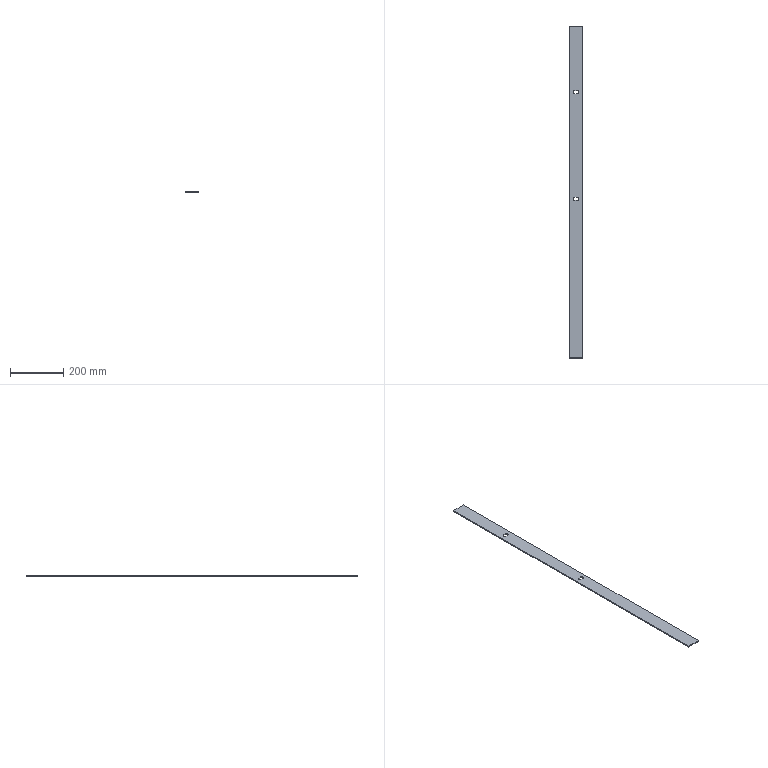Part | STEP file | E3-护栏加固Plate 1 | 1 solid | 16 faces | box 52 x 1250 x 4 mm | volume 258135 mm3 | plane 10 | cylinder 6 | commonest cylinder face diameters 12 x6
STEP:
#1=CARTESIAN_POINT('',(0.,0.,0.));
#2=DIRECTION('',(0.,0.,1.));
#3=DIRECTION('',(1.,0.,0.));
#4=AXIS2_PLACEMENT_3D('',#1,#2,#3);
#5=CARTESIAN_POINT('',(5.,369.,-4.));
#6=VERTEX_POINT('',#5);
#7=CARTESIAN_POINT('',(5.,369.,0.));
#8=VERTEX_POINT('',#7);
#9=CARTESIAN_POINT('',(5.,369.,-4.));
#10=DIRECTION('',(0.,0.,1.));
#11=VECTOR('',#10,1.);
#12=LINE('',#9,#11);
#13=CARTESIAN_POINT('',(5.,375.,-4.));
#14=DIRECTION('',(0.,0.,-1.));
#15=DIRECTION('',(1.,0.,0.));
#16=AXIS2_PLACEMENT_3D('',#13,#14,#15);
#17=CYLINDRICAL_SURFACE('',#16,6.);
#18=CARTESIAN_POINT('',(1.571,0.));
#19=DIRECTION('',(0.,-1.));
#20=VECTOR('',#19,1.);
#21=LINE('',#18,#20);
#22=(GEOMETRIC_REPRESENTATION_CONTEXT(2)PARAMETRIC_REPRESENTATION_CONTEXT()REPRESENTATION_CONTEXT('',''));
#23=DEFINITIONAL_REPRESENTATION('',(#21),#22);
#24=PCURVE('',#17,#23);
#25=CARTESIAN_POINT('',(-5.,369.,-4.));
#26=DIRECTION('',(0.,-1.,0.));
#27=DIRECTION('',(0.,0.,1.));
#28=AXIS2_PLACEMENT_3D('',#25,#26,#27);
#29=PLANE('',#28);
#30=CARTESIAN_POINT('',(0.,-10.));
#31=DIRECTION('',(1.,0.));
#32=VECTOR('',#31,1.);
#33=LINE('',#30,#32);
#34=(GEOMETRIC_REPRESENTATION_CONTEXT(2)PARAMETRIC_REPRESENTATION_CONTEXT()REPRESENTATION_CONTEXT('',''));
#35=DEFINITIONAL_REPRESENTATION('',(#33),#34);
#36=PCURVE('',#29,#35);
#37=SURFACE_CURVE('',#12,(#24,#36),.PCURVE_S1.);
#38=EDGE_CURVE('',#6,#8,#37,.T.);
#39=ORIENTED_EDGE('',*,*,#38,.F.);
#40=CARTESIAN_POINT('',(11.,375.,-4.));
#41=VERTEX_POINT('',#40);
#42=CARTESIAN_POINT('',(5.,375.,-4.));
#43=DIRECTION('',(0.,0.,1.));
#44=DIRECTION('',(1.,0.,0.));
#45=AXIS2_PLACEMENT_3D('',#42,#43,#44);
#46=CIRCLE('',#45,6.);
#47=CARTESIAN_POINT('',(6.283,0.));
#48=DIRECTION('',(-1.,0.));
#49=VECTOR('',#48,1.);
#50=LINE('',#47,#49);
#51=(GEOMETRIC_REPRESENTATION_CONTEXT(2)PARAMETRIC_REPRESENTATION_CONTEXT()REPRESENTATION_CONTEXT('',''));
#52=DEFINITIONAL_REPRESENTATION('',(#50),#51);
#53=PCURVE('',#17,#52);
#54=CARTESIAN_POINT('',(0.,0.,-4.));
#55=DIRECTION('',(0.,0.,-1.));
#56=DIRECTION('',(1.,0.,0.));
#57=AXIS2_PLACEMENT_3D('',#54,#55,#56);
#58=PLANE('',#57);
#59=CARTESIAN_POINT('',(11.,-375.));
#60=CARTESIAN_POINT('',(11.,-385.392));
#61=CARTESIAN_POINT('',(2.,-380.196));
#62=CARTESIAN_POINT('',(-7.,-375.));
#63=CARTESIAN_POINT('',(2.,-369.804));
#64=CARTESIAN_POINT('',(11.,-364.608));
#65=CARTESIAN_POINT('',(11.,-375.));
#66=(BOUNDED_CURVE()B_SPLINE_CURVE(2,(#59,#60,#61,#62,#63,#64,#65),.UNSPECIFIED.,.T.,.F.)B_SPLINE_CURVE_WITH_KNOTS((1,2,2,2,2,1),(-2.094,0.,2.094,4.189,6.283,8.378),.UNSPECIFIED.)CURVE()GEOMETRIC_REPRESENTATION_ITEM()RATIONAL_B_SPLINE_CURVE((1.,0.5,1.,0.5,1.,0.5,1.))REPRESENTATION_ITEM(''));
#67=(GEOMETRIC_REPRESENTATION_CONTEXT(2)PARAMETRIC_REPRESENTATION_CONTEXT()REPRESENTATION_CONTEXT('',''));
#68=DEFINITIONAL_REPRESENTATION('',(#66),#67);
#69=PCURVE('',#58,#68);
#70=SURFACE_CURVE('',#46,(#53,#69),.PCURVE_S1.);
#71=EDGE_CURVE('',#6,#41,#70,.T.);
#72=ORIENTED_EDGE('',*,*,#71,.T.);
#73=CARTESIAN_POINT('',(11.,375.,0.));
#74=VERTEX_POINT('',#73);
#75=CARTESIAN_POINT('',(11.,375.,-4.));
#76=DIRECTION('',(0.,0.,-1.));
#77=VECTOR('',#76,1.);
#78=LINE('',#75,#77);
#79=CARTESIAN_POINT('',(0.,0.));
#80=DIRECTION('',(0.,1.));
#81=VECTOR('',#80,1.);
#82=LINE('',#79,#81);
#83=(GEOMETRIC_REPRESENTATION_CONTEXT(2)PARAMETRIC_REPRESENTATION_CONTEXT()REPRESENTATION_CONTEXT('',''));
#84=DEFINITIONAL_REPRESENTATION('',(#82),#83);
#85=PCURVE('',#17,#84);
#86=CARTESIAN_POINT('',(5.,375.,-4.));
#87=DIRECTION('',(0.,0.,-1.));
#88=DIRECTION('',(1.,0.,0.));
#89=AXIS2_PLACEMENT_3D('',#86,#87,#88);
#90=CYLINDRICAL_SURFACE('',#89,6.);
#91=CARTESIAN_POINT('',(6.283,0.));
#92=DIRECTION('',(0.,1.));
#93=VECTOR('',#92,1.);
#94=LINE('',#91,#93);
#95=(GEOMETRIC_REPRESENTATION_CONTEXT(2)PARAMETRIC_REPRESENTATION_CONTEXT()REPRESENTATION_CONTEXT('',''));
#96=DEFINITIONAL_REPRESENTATION('',(#94),#95);
#97=PCURVE('',#90,#96);
#98=SURFACE_CURVE('',#78,(#85,#97),.PCURVE_S1.);
#99=EDGE_CURVE('',#74,#41,#98,.T.);
#100=ORIENTED_EDGE('',*,*,#99,.F.);
#101=CARTESIAN_POINT('',(5.,375.,0.));
#102=DIRECTION('',(0.,0.,1.));
#103=DIRECTION('',(1.,0.,0.));
#104=AXIS2_PLACEMENT_3D('',#101,#102,#103);
#105=CIRCLE('',#104,6.);
#106=CARTESIAN_POINT('',(6.283,-4.));
#107=DIRECTION('',(-1.,0.));
#108=VECTOR('',#107,1.);
#109=LINE('',#106,#108);
#110=(GEOMETRIC_REPRESENTATION_CONTEXT(2)PARAMETRIC_REPRESENTATION_CONTEXT()REPRESENTATION_CONTEXT('',''));
#111=DEFINITIONAL_REPRESENTATION('',(#109),#110);
#112=PCURVE('',#17,#111);
#113=CARTESIAN_POINT('',(0.,0.,0.));
#114=DIRECTION('',(0.,0.,-1.));
#115=DIRECTION('',(1.,0.,0.));
#116=AXIS2_PLACEMENT_3D('',#113,#114,#115);
#117=PLANE('',#116);
#118=CARTESIAN_POINT('',(11.,-375.));
#119=CARTESIAN_POINT('',(11.,-385.392));
#120=CARTESIAN_POINT('',(2.,-380.196));
#121=CARTESIAN_POINT('',(-7.,-375.));
#122=CARTESIAN_POINT('',(2.,-369.804));
#123=CARTESIAN_POINT('',(11.,-364.608));
#124=CARTESIAN_POINT('',(11.,-375.));
#125=(BOUNDED_CURVE()B_SPLINE_CURVE(2,(#118,#119,#120,#121,#122,#123,#124),.UNSPECIFIED.,.T.,.F.)B_SPLINE_CURVE_WITH_KNOTS((1,2,2,2,2,1),(-2.094,0.,2.094,4.189,6.283,8.378),.UNSPECIFIED.)CURVE()GEOMETRIC_REPRESENTATION_ITEM()RATIONAL_B_SPLINE_CURVE((1.,0.5,1.,0.5,1.,0.5,1.))REPRESENTATION_ITEM(''));
#126=(GEOMETRIC_REPRESENTATION_CONTEXT(2)PARAMETRIC_REPRESENTATION_CONTEXT()REPRESENTATION_CONTEXT('',''));
#127=DEFINITIONAL_REPRESENTATION('',(#125),#126);
#128=PCURVE('',#117,#127);
#129=SURFACE_CURVE('',#105,(#112,#128),.PCURVE_S1.);
#130=EDGE_CURVE('',#8,#74,#129,.T.);
#131=ORIENTED_EDGE('',*,*,#130,.F.);
#132=EDGE_LOOP('',(#39,#72,#100,#131));
#133=FACE_BOUND('',#132,.F.);
#134=ADVANCED_FACE('',(#133),#17,.F.);
#135=CARTESIAN_POINT('',(5.,-31.,-4.));
#136=VERTEX_POINT('',#135);
#137=CARTESIAN_POINT('',(5.,-31.,0.));
#138=VERTEX_POINT('',#137);
#139=CARTESIAN_POINT('',(5.,-31.,-4.));
#140=DIRECTION('',(0.,0.,1.));
#141=VECTOR('',#140,1.);
#142=LINE('',#139,#141);
#143=CARTESIAN_POINT('',(5.,-25.,-4.));
#144=DIRECTION('',(0.,0.,-1.));
#145=DIRECTION('',(1.,0.,0.));
#146=AXIS2_PLACEMENT_3D('',#143,#144,#145);
#147=CYLINDRICAL_SURFACE('',#146,6.);
#148=CARTESIAN_POINT('',(1.571,0.));
#149=DIRECTION('',(0.,-1.));
#150=VECTOR('',#149,1.);
#151=LINE('',#148,#150);
#152=(GEOMETRIC_REPRESENTATION_CONTEXT(2)PARAMETRIC_REPRESENTATION_CONTEXT()REPRESENTATION_CONTEXT('',''));
#153=DEFINITIONAL_REPRESENTATION('',(#151),#152);
#154=PCURVE('',#147,#153);
#155=CARTESIAN_POINT('',(-5.,-31.,-4.));
#156=DIRECTION('',(0.,-1.,0.));
#157=DIRECTION('',(0.,0.,1.));
#158=AXIS2_PLACEMENT_3D('',#155,#156,#157);
#159=PLANE('',#158);
#160=CARTESIAN_POINT('',(0.,-10.));
#161=DIRECTION('',(1.,0.));
#162=VECTOR('',#161,1.);
#163=LINE('',#160,#162);
#164=(GEOMETRIC_REPRESENTATION_CONTEXT(2)PARAMETRIC_REPRESENTATION_CONTEXT()REPRESENTATION_CONTEXT('',''));
#165=DEFINITIONAL_REPRESENTATION('',(#163),#164);
#166=PCURVE('',#159,#165);
#167=SURFACE_CURVE('',#142,(#154,#166),.PCURVE_S1.);
#168=EDGE_CURVE('',#136,#138,#167,.T.);
#169=ORIENTED_EDGE('',*,*,#168,.F.);
#170=CARTESIAN_POINT('',(11.,-25.,-4.));
#171=VERTEX_POINT('',#170);
#172=CARTESIAN_POINT('',(5.,-25.,-4.));
#173=DIRECTION('',(0.,0.,1.));
#174=DIRECTION('',(1.,0.,0.));
#175=AXIS2_PLACEMENT_3D('',#172,#173,#174);
#176=CIRCLE('',#175,6.);
#177=CARTESIAN_POINT('',(6.283,0.));
#178=DIRECTION('',(-1.,0.));
#179=VECTOR('',#178,1.);
#180=LINE('',#177,#179);
#181=(GEOMETRIC_REPRESENTATION_CONTEXT(2)PARAMETRIC_REPRESENTATION_CONTEXT()REPRESENTATION_CONTEXT('',''));
#182=DEFINITIONAL_REPRESENTATION('',(#180),#181);
#183=PCURVE('',#147,#182);
#184=CARTESIAN_POINT('',(11.,25.));
#185=CARTESIAN_POINT('',(11.,14.608));
#186=CARTESIAN_POINT('',(2.,19.804));
#187=CARTESIAN_POINT('',(-7.,25.));
#188=CARTESIAN_POINT('',(2.,30.196));
#189=CARTESIAN_POINT('',(11.,35.392));
#190=CARTESIAN_POINT('',(11.,25.));
#191=(BOUNDED_CURVE()B_SPLINE_CURVE(2,(#184,#185,#186,#187,#188,#189,#190),.UNSPECIFIED.,.T.,.F.)B_SPLINE_CURVE_WITH_KNOTS((1,2,2,2,2,1),(-2.094,0.,2.094,4.189,6.283,8.378),.UNSPECIFIED.)CURVE()GEOMETRIC_REPRESENTATION_ITEM()RATIONAL_B_SPLINE_CURVE((1.,0.5,1.,0.5,1.,0.5,1.))REPRESENTATION_ITEM(''));
#192=(GEOMETRIC_REPRESENTATION_CONTEXT(2)PARAMETRIC_REPRESENTATION_CONTEXT()REPRESENTATION_CONTEXT('',''));
#193=DEFINITIONAL_REPRESENTATION('',(#191),#192);
#194=PCURVE('',#58,#193);
#195=SURFACE_CURVE('',#176,(#183,#194),.PCURVE_S1.);
#196=EDGE_CURVE('',#136,#171,#195,.T.);
#197=ORIENTED_EDGE('',*,*,#196,.T.);
#198=CARTESIAN_POINT('',(11.,-25.,0.));
#199=VERTEX_POINT('',#198);
#200=CARTESIAN_POINT('',(11.,-25.,-4.));
#201=DIRECTION('',(0.,0.,-1.));
#202=VECTOR('',#201,1.);
#203=LINE('',#200,#202);
#204=CARTESIAN_POINT('',(0.,0.));
#205=DIRECTION('',(0.,1.));
#206=VECTOR('',#205,1.);
#207=LINE('',#204,#206);
#208=(GEOMETRIC_REPRESENTATION_CONTEXT(2)PARAMETRIC_REPRESENTATION_CONTEXT()REPRESENTATION_CONTEXT('',''));
#209=DEFINITIONAL_REPRESENTATION('',(#207),#208);
#210=PCURVE('',#147,#209);
#211=CARTESIAN_POINT('',(5.,-25.,-4.));
#212=DIRECTION('',(0.,0.,-1.));
#213=DIRECTION('',(1.,0.,0.));
#214=AXIS2_PLACEMENT_3D('',#211,#212,#213);
#215=CYLINDRICAL_SURFACE('',#214,6.);
#216=CARTESIAN_POINT('',(6.283,0.));
#217=DIRECTION('',(0.,1.));
#218=VECTOR('',#217,1.);
#219=LINE('',#216,#218);
#220=(GEOMETRIC_REPRESENTATION_CONTEXT(2)PARAMETRIC_REPRESENTATION_CONTEXT()REPRESENTATION_CONTEXT('',''));
#221=DEFINITIONAL_REPRESENTATION('',(#219),#220);
#222=PCURVE('',#215,#221);
#223=SURFACE_CURVE('',#203,(#210,#222),.PCURVE_S1.);
#224=EDGE_CURVE('',#199,#171,#223,.T.);
#225=ORIENTED_EDGE('',*,*,#224,.F.);
#226=CARTESIAN_POINT('',(5.,-25.,0.));
#227=DIRECTION('',(0.,0.,1.));
#228=DIRECTION('',(1.,0.,0.));
#229=AXIS2_PLACEMENT_3D('',#226,#227,#228);
#230=CIRCLE('',#229,6.);
#231=CARTESIAN_POINT('',(6.283,-4.));
#232=DIRECTION('',(-1.,0.));
#233=VECTOR('',#232,1.);
#234=LINE('',#231,#233);
#235=(GEOMETRIC_REPRESENTATION_CONTEXT(2)PARAMETRIC_REPRESENTATION_CONTEXT()REPRESENTATION_CONTEXT('',''));
#236=DEFINITIONAL_REPRESENTATION('',(#234),#235);
#237=PCURVE('',#147,#236);
#238=CARTESIAN_POINT('',(11.,25.));
#239=CARTESIAN_POINT('',(11.,14.608));
#240=CARTESIAN_POINT('',(2.,19.804));
#241=CARTESIAN_POINT('',(-7.,25.));
#242=CARTESIAN_POINT('',(2.,30.196));
#243=CARTESIAN_POINT('',(11.,35.392));
#244=CARTESIAN_POINT('',(11.,25.));
#245=(BOUNDED_CURVE()B_SPLINE_CURVE(2,(#238,#239,#240,#241,#242,#243,#244),.UNSPECIFIED.,.T.,.F.)B_SPLINE_CURVE_WITH_KNOTS((1,2,2,2,2,1),(-2.094,0.,2.094,4.189,6.283,8.378),.UNSPECIFIED.)CURVE()GEOMETRIC_REPRESENTATION_ITEM()RATIONAL_B_SPLINE_CURVE((1.,0.5,1.,0.5,1.,0.5,1.))REPRESENTATION_ITEM(''));
#246=(GEOMETRIC_REPRESENTATION_CONTEXT(2)PARAMETRIC_REPRESENTATION_CONTEXT()REPRESENTATION_CONTEXT('',''));
#247=DEFINITIONAL_REPRESENTATION('',(#245),#246);
#248=PCURVE('',#117,#247);
#249=SURFACE_CURVE('',#230,(#237,#248),.PCURVE_S1.);
#250=EDGE_CURVE('',#138,#199,#249,.T.);
#251=ORIENTED_EDGE('',*,*,#250,.F.);
#252=EDGE_LOOP('',(#169,#197,#225,#251));
#253=FACE_BOUND('',#252,.F.);
#254=ADVANCED_FACE('',(#253),#147,.F.);
#255=CARTESIAN_POINT('',(-5.,-19.,0.));
#256=VERTEX_POINT('',#255);
#257=CARTESIAN_POINT('',(5.,-19.,0.));
#258=VERTEX_POINT('',#257);
#259=CARTESIAN_POINT('',(-5.,-19.,0.));
#260=DIRECTION('',(1.,0.,0.));
#261=VECTOR('',#260,1.);
#262=LINE('',#259,#261);
#263=CARTESIAN_POINT('',(-5.,19.));
#264=DIRECTION('',(1.,0.));
#265=VECTOR('',#264,1.);
#266=LINE('',#263,#265);
#267=(GEOMETRIC_REPRESENTATION_CONTEXT(2)PARAMETRIC_REPRESENTATION_CONTEXT()REPRESENTATION_CONTEXT('',''));
#268=DEFINITIONAL_REPRESENTATION('',(#266),#267);
#269=PCURVE('',#117,#268);
#270=CARTESIAN_POINT('',(-5.,-19.,-4.));
#271=DIRECTION('',(0.,1.,0.));
#272=DIRECTION('',(0.,0.,-1.));
#273=AXIS2_PLACEMENT_3D('',#270,#271,#272);
#274=PLANE('',#273);
#275=CARTESIAN_POINT('',(-4.,0.));
#276=DIRECTION('',(0.,-1.));
#277=VECTOR('',#276,1.);
#278=LINE('',#275,#277);
#279=(GEOMETRIC_REPRESENTATION_CONTEXT(2)PARAMETRIC_REPRESENTATION_CONTEXT()REPRESENTATION_CONTEXT('',''));
#280=DEFINITIONAL_REPRESENTATION('',(#278),#279);
#281=PCURVE('',#274,#280);
#282=SURFACE_CURVE('',#262,(#269,#281),.PCURVE_S1.);
#283=EDGE_CURVE('',#256,#258,#282,.T.);
#284=ORIENTED_EDGE('',*,*,#283,.T.);
#285=CARTESIAN_POINT('',(5.,-25.,0.));
#286=DIRECTION('',(0.,0.,1.));
#287=DIRECTION('',(1.,0.,0.));
#288=AXIS2_PLACEMENT_3D('',#285,#286,#287);
#289=CIRCLE('',#288,6.);
#290=CARTESIAN_POINT('',(11.,25.));
#291=CARTESIAN_POINT('',(11.,14.608));
#292=CARTESIAN_POINT('',(2.,19.804));
#293=CARTESIAN_POINT('',(-7.,25.));
#294=CARTESIAN_POINT('',(2.,30.196));
#295=CARTESIAN_POINT('',(11.,35.392));
#296=CARTESIAN_POINT('',(11.,25.));
#297=(BOUNDED_CURVE()B_SPLINE_CURVE(2,(#290,#291,#292,#293,#294,#295,#296),.UNSPECIFIED.,.T.,.F.)B_SPLINE_CURVE_WITH_KNOTS((1,2,2,2,2,1),(-2.094,0.,2.094,4.189,6.283,8.378),.UNSPECIFIED.)CURVE()GEOMETRIC_REPRESENTATION_ITEM()RATIONAL_B_SPLINE_CURVE((1.,0.5,1.,0.5,1.,0.5,1.))REPRESENTATION_ITEM(''));
#298=(GEOMETRIC_REPRESENTATION_CONTEXT(2)PARAMETRIC_REPRESENTATION_CONTEXT()REPRESENTATION_CONTEXT('',''));
#299=DEFINITIONAL_REPRESENTATION('',(#297),#298);
#300=PCURVE('',#117,#299);
#301=CARTESIAN_POINT('',(6.283,-4.));
#302=DIRECTION('',(-1.,0.));
#303=VECTOR('',#302,1.);
#304=LINE('',#301,#303);
#305=(GEOMETRIC_REPRESENTATION_CONTEXT(2)PARAMETRIC_REPRESENTATION_CONTEXT()REPRESENTATION_CONTEXT('',''));
#306=DEFINITIONAL_REPRESENTATION('',(#304),#305);
#307=PCURVE('',#215,#306);
#308=SURFACE_CURVE('',#289,(#300,#307),.PCURVE_S1.);
#309=EDGE_CURVE('',#199,#258,#308,.T.);
#310=ORIENTED_EDGE('',*,*,#309,.F.);
#311=ORIENTED_EDGE('',*,*,#250,.F.);
#312=CARTESIAN_POINT('',(-5.,-31.,0.));
#313=VERTEX_POINT('',#312);
#314=CARTESIAN_POINT('',(-5.,-31.,0.));
#315=DIRECTION('',(1.,0.,0.));
#316=VECTOR('',#315,1.);
#317=LINE('',#314,#316);
#318=CARTESIAN_POINT('',(-5.,31.));
#319=DIRECTION('',(1.,0.));
#320=VECTOR('',#319,1.);
#321=LINE('',#318,#320);
#322=(GEOMETRIC_REPRESENTATION_CONTEXT(2)PARAMETRIC_REPRESENTATION_CONTEXT()REPRESENTATION_CONTEXT('',''));
#323=DEFINITIONAL_REPRESENTATION('',(#321),#322);
#324=PCURVE('',#117,#323);
#325=CARTESIAN_POINT('',(4.,0.));
#326=DIRECTION('',(0.,-1.));
#327=VECTOR('',#326,1.);
#328=LINE('',#325,#327);
#329=(GEOMETRIC_REPRESENTATION_CONTEXT(2)PARAMETRIC_REPRESENTATION_CONTEXT()REPRESENTATION_CONTEXT('',''));
#330=DEFINITIONAL_REPRESENTATION('',(#328),#329);
#331=PCURVE('',#159,#330);
#332=SURFACE_CURVE('',#317,(#324,#331),.PCURVE_S1.);
#333=EDGE_CURVE('',#313,#138,#332,.T.);
#334=ORIENTED_EDGE('',*,*,#333,.F.);
#335=CARTESIAN_POINT('',(-5.,-25.,0.));
#336=DIRECTION('',(0.,0.,1.));
#337=DIRECTION('',(1.,0.,0.));
#338=AXIS2_PLACEMENT_3D('',#335,#336,#337);
#339=CIRCLE('',#338,6.);
#340=CARTESIAN_POINT('',(1.,25.));
#341=CARTESIAN_POINT('',(1.,14.608));
#342=CARTESIAN_POINT('',(-8.,19.804));
#343=CARTESIAN_POINT('',(-17.,25.));
#344=CARTESIAN_POINT('',(-8.,30.196));
#345=CARTESIAN_POINT('',(1.,35.392));
#346=CARTESIAN_POINT('',(1.,25.));
#347=(BOUNDED_CURVE()B_SPLINE_CURVE(2,(#340,#341,#342,#343,#344,#345,#346),.UNSPECIFIED.,.T.,.F.)B_SPLINE_CURVE_WITH_KNOTS((1,2,2,2,2,1),(-2.094,0.,2.094,4.189,6.283,8.378),.UNSPECIFIED.)CURVE()GEOMETRIC_REPRESENTATION_ITEM()RATIONAL_B_SPLINE_CURVE((1.,0.5,1.,0.5,1.,0.5,1.))REPRESENTATION_ITEM(''));
#348=(GEOMETRIC_REPRESENTATION_CONTEXT(2)PARAMETRIC_REPRESENTATION_CONTEXT()REPRESENTATION_CONTEXT('',''));
#349=DEFINITIONAL_REPRESENTATION('',(#347),#348);
#350=PCURVE('',#117,#349);
#351=CARTESIAN_POINT('',(-5.,-25.,-4.));
#352=DIRECTION('',(0.,0.,-1.));
#353=DIRECTION('',(1.,0.,0.));
#354=AXIS2_PLACEMENT_3D('',#351,#352,#353);
#355=CYLINDRICAL_SURFACE('',#354,6.);
#356=CARTESIAN_POINT('',(6.283,-4.));
#357=DIRECTION('',(-1.,0.));
#358=VECTOR('',#357,1.);
#359=LINE('',#356,#358);
#360=(GEOMETRIC_REPRESENTATION_CONTEXT(2)PARAMETRIC_REPRESENTATION_CONTEXT()REPRESENTATION_CONTEXT('',''));
#361=DEFINITIONAL_REPRESENTATION('',(#359),#360);
#362=PCURVE('',#355,#361);
#363=SURFACE_CURVE('',#339,(#350,#362),.PCURVE_S1.);
#364=EDGE_CURVE('',#256,#313,#363,.T.);
#365=ORIENTED_EDGE('',*,*,#364,.F.);
#366=EDGE_LOOP('',(#284,#310,#311,#334,#365));
#367=FACE_BOUND('',#366,.T.);
#368=CARTESIAN_POINT('',(26.,-625.,0.));
#369=VERTEX_POINT('',#368);
#370=CARTESIAN_POINT('',(26.,625.,0.));
#371=VERTEX_POINT('',#370);
#372=CARTESIAN_POINT('',(26.,625.,0.));
#373=DIRECTION('',(0.,1.,0.));
#374=VECTOR('',#373,1.);
#375=LINE('',#372,#374);
#376=CARTESIAN_POINT('',(26.,-625.));
#377=DIRECTION('',(0.,-1.));
#378=VECTOR('',#377,1.);
#379=LINE('',#376,#378);
#380=(GEOMETRIC_REPRESENTATION_CONTEXT(2)PARAMETRIC_REPRESENTATION_CONTEXT()REPRESENTATION_CONTEXT('',''));
#381=DEFINITIONAL_REPRESENTATION('',(#379),#380);
#382=PCURVE('',#117,#381);
#383=CARTESIAN_POINT('',(26.,625.,-4.));
#384=DIRECTION('',(-1.,0.,0.));
#385=DIRECTION('',(0.,-1.,0.));
#386=AXIS2_PLACEMENT_3D('',#383,#384,#385);
#387=PLANE('',#386);
#388=CARTESIAN_POINT('',(0.,4.));
#389=DIRECTION('',(-1.,0.));
#390=VECTOR('',#389,1.);
#391=LINE('',#388,#390);
#392=(GEOMETRIC_REPRESENTATION_CONTEXT(2)PARAMETRIC_REPRESENTATION_CONTEXT()REPRESENTATION_CONTEXT('',''));
#393=DEFINITIONAL_REPRESENTATION('',(#391),#392);
#394=PCURVE('',#387,#393);
#395=SURFACE_CURVE('',#375,(#382,#394),.PCURVE_S1.);
#396=EDGE_CURVE('',#369,#371,#395,.T.);
#397=ORIENTED_EDGE('',*,*,#396,.T.);
#398=CARTESIAN_POINT('',(-26.,625.,0.));
#399=VERTEX_POINT('',#398);
#400=CARTESIAN_POINT('',(-26.,625.,0.));
#401=DIRECTION('',(-1.,0.,0.));
#402=VECTOR('',#401,1.);
#403=LINE('',#400,#402);
#404=CARTESIAN_POINT('',(-26.,-625.));
#405=DIRECTION('',(-1.,0.));
#406=VECTOR('',#405,1.);
#407=LINE('',#404,#406);
#408=(GEOMETRIC_REPRESENTATION_CONTEXT(2)PARAMETRIC_REPRESENTATION_CONTEXT()REPRESENTATION_CONTEXT('',''));
#409=DEFINITIONAL_REPRESENTATION('',(#407),#408);
#410=PCURVE('',#117,#409);
#411=CARTESIAN_POINT('',(-26.,625.,-4.));
#412=DIRECTION('',(0.,-1.,0.));
#413=DIRECTION('',(0.,0.,1.));
#414=AXIS2_PLACEMENT_3D('',#411,#412,#413);
#415=PLANE('',#414);
#416=CARTESIAN_POINT('',(4.,0.));
#417=DIRECTION('',(0.,1.));
#418=VECTOR('',#417,1.);
#419=LINE('',#416,#418);
#420=(GEOMETRIC_REPRESENTATION_CONTEXT(2)PARAMETRIC_REPRESENTATION_CONTEXT()REPRESENTATION_CONTEXT('',''));
#421=DEFINITIONAL_REPRESENTATION('',(#419),#420);
#422=PCURVE('',#415,#421);
#423=SURFACE_CURVE('',#403,(#410,#422),.PCURVE_S1.);
#424=EDGE_CURVE('',#371,#399,#423,.T.);
#425=ORIENTED_EDGE('',*,*,#424,.T.);
#426=CARTESIAN_POINT('',(-26.,-625.,0.));
#427=VERTEX_POINT('',#426);
#428=CARTESIAN_POINT('',(-26.,625.,0.));
#429=DIRECTION('',(0.,-1.,0.));
#430=VECTOR('',#429,1.);
#431=LINE('',#428,#430);
#432=CARTESIAN_POINT('',(-26.,-625.));
#433=DIRECTION('',(0.,1.));
#434=VECTOR('',#433,1.);
#435=LINE('',#432,#434);
#436=(GEOMETRIC_REPRESENTATION_CONTEXT(2)PARAMETRIC_REPRESENTATION_CONTEXT()REPRESENTATION_CONTEXT('',''));
#437=DEFINITIONAL_REPRESENTATION('',(#435),#436);
#438=PCURVE('',#117,#437);
#439=CARTESIAN_POINT('',(-26.,625.,-4.));
#440=DIRECTION('',(1.,0.,0.));
#441=DIRECTION('',(0.,1.,0.));
#442=AXIS2_PLACEMENT_3D('',#439,#440,#441);
#443=PLANE('',#442);
#444=CARTESIAN_POINT('',(0.,4.));
#445=DIRECTION('',(-1.,0.));
#446=VECTOR('',#445,1.);
#447=LINE('',#444,#446);
#448=(GEOMETRIC_REPRESENTATION_CONTEXT(2)PARAMETRIC_REPRESENTATION_CONTEXT()REPRESENTATION_CONTEXT('',''));
#449=DEFINITIONAL_REPRESENTATION('',(#447),#448);
#450=PCURVE('',#443,#449);
#451=SURFACE_CURVE('',#431,(#438,#450),.PCURVE_S1.);
#452=EDGE_CURVE('',#399,#427,#451,.T.);
#453=ORIENTED_EDGE('',*,*,#452,.T.);
#454=CARTESIAN_POINT('',(-26.,-625.,0.));
#455=DIRECTION('',(1.,0.,0.));
#456=VECTOR('',#455,1.);
#457=LINE('',#454,#456);
#458=CARTESIAN_POINT('',(-26.,625.));
#459=DIRECTION('',(1.,0.));
#460=VECTOR('',#459,1.);
#461=LINE('',#458,#460);
#462=(GEOMETRIC_REPRESENTATION_CONTEXT(2)PARAMETRIC_REPRESENTATION_CONTEXT()REPRESENTATION_CONTEXT('',''));
#463=DEFINITIONAL_REPRESENTATION('',(#461),#462);
#464=PCURVE('',#117,#463);
#465=CARTESIAN_POINT('',(-26.,-625.,-4.));
#466=DIRECTION('',(0.,1.,0.));
#467=DIRECTION('',(0.,0.,-1.));
#468=AXIS2_PLACEMENT_3D('',#465,#466,#467);
#469=PLANE('',#468);
#470=CARTESIAN_POINT('',(-4.,0.));
#471=DIRECTION('',(0.,-1.));
#472=VECTOR('',#471,1.);
#473=LINE('',#470,#472);
#474=(GEOMETRIC_REPRESENTATION_CONTEXT(2)PARAMETRIC_REPRESENTATION_CONTEXT()REPRESENTATION_CONTEXT('',''));
#475=DEFINITIONAL_REPRESENTATION('',(#473),#474);
#476=PCURVE('',#469,#475);
#477=SURFACE_CURVE('',#457,(#464,#476),.PCURVE_S1.);
#478=EDGE_CURVE('',#427,#369,#477,.T.);
#479=ORIENTED_EDGE('',*,*,#478,.T.);
#480=EDGE_LOOP('',(#397,#425,#453,#479));
#481=FACE_BOUND('',#480,.T.);
#482=CARTESIAN_POINT('',(-5.,381.,0.));
#483=VERTEX_POINT('',#482);
#484=CARTESIAN_POINT('',(5.,381.,0.));
#485=VERTEX_POINT('',#484);
#486=CARTESIAN_POINT('',(-5.,381.,0.));
#487=DIRECTION('',(1.,0.,0.));
#488=VECTOR('',#487,1.);
#489=LINE('',#486,#488);
#490=CARTESIAN_POINT('',(-5.,-381.));
#491=DIRECTION('',(1.,0.));
#492=VECTOR('',#491,1.);
#493=LINE('',#490,#492);
#494=(GEOMETRIC_REPRESENTATION_CONTEXT(2)PARAMETRIC_REPRESENTATION_CONTEXT()REPRESENTATION_CONTEXT('',''));
#495=DEFINITIONAL_REPRESENTATION('',(#493),#494);
#496=PCURVE('',#117,#495);
#497=CARTESIAN_POINT('',(-5.,381.,-4.));
#498=DIRECTION('',(0.,1.,0.));
#499=DIRECTION('',(0.,0.,-1.));
#500=AXIS2_PLACEMENT_3D('',#497,#498,#499);
#501=PLANE('',#500);
#502=CARTESIAN_POINT('',(-4.,0.));
#503=DIRECTION('',(0.,-1.));
#504=VECTOR('',#503,1.);
#505=LINE('',#502,#504);
#506=(GEOMETRIC_REPRESENTATION_CONTEXT(2)PARAMETRIC_REPRESENTATION_CONTEXT()REPRESENTATION_CONTEXT('',''));
#507=DEFINITIONAL_REPRESENTATION('',(#505),#506);
#508=PCURVE('',#501,#507);
#509=SURFACE_CURVE('',#489,(#496,#508),.PCURVE_S1.);
#510=EDGE_CURVE('',#483,#485,#509,.T.);
#511=ORIENTED_EDGE('',*,*,#510,.T.);
#512=CARTESIAN_POINT('',(5.,375.,0.));
#513=DIRECTION('',(0.,0.,1.));
#514=DIRECTION('',(1.,0.,0.));
#515=AXIS2_PLACEMENT_3D('',#512,#513,#514);
#516=CIRCLE('',#515,6.);
#517=CARTESIAN_POINT('',(11.,-375.));
#518=CARTESIAN_POINT('',(11.,-385.392));
#519=CARTESIAN_POINT('',(2.,-380.196));
#520=CARTESIAN_POINT('',(-7.,-375.));
#521=CARTESIAN_POINT('',(2.,-369.804));
#522=CARTESIAN_POINT('',(11.,-364.608));
#523=CARTESIAN_POINT('',(11.,-375.));
#524=(BOUNDED_CURVE()B_SPLINE_CURVE(2,(#517,#518,#519,#520,#521,#522,#523),.UNSPECIFIED.,.T.,.F.)B_SPLINE_CURVE_WITH_KNOTS((1,2,2,2,2,1),(-2.094,0.,2.094,4.189,6.283,8.378),.UNSPECIFIED.)CURVE()GEOMETRIC_REPRESENTATION_ITEM()RATIONAL_B_SPLINE_CURVE((1.,0.5,1.,0.5,1.,0.5,1.))REPRESENTATION_ITEM(''));
#525=(GEOMETRIC_REPRESENTATION_CONTEXT(2)PARAMETRIC_REPRESENTATION_CONTEXT()REPRESENTATION_CONTEXT('',''));
#526=DEFINITIONAL_REPRESENTATION('',(#524),#525);
#527=PCURVE('',#117,#526);
#528=CARTESIAN_POINT('',(6.283,-4.));
#529=DIRECTION('',(-1.,0.));
#530=VECTOR('',#529,1.);
#531=LINE('',#528,#530);
#532=(GEOMETRIC_REPRESENTATION_CONTEXT(2)PARAMETRIC_REPRESENTATION_CONTEXT()REPRESENTATION_CONTEXT('',''));
#533=DEFINITIONAL_REPRESENTATION('',(#531),#532);
#534=PCURVE('',#90,#533);
#535=SURFACE_CURVE('',#516,(#527,#534),.PCURVE_S1.);
#536=EDGE_CURVE('',#74,#485,#535,.T.);
#537=ORIENTED_EDGE('',*,*,#536,.F.);
#538=ORIENTED_EDGE('',*,*,#130,.F.);
#539=CARTESIAN_POINT('',(-5.,369.,0.));
#540=VERTEX_POINT('',#539);
#541=CARTESIAN_POINT('',(-5.,369.,0.));
#542=DIRECTION('',(1.,0.,0.));
#543=VECTOR('',#542,1.);
#544=LINE('',#541,#543);
#545=CARTESIAN_POINT('',(-5.,-369.));
#546=DIRECTION('',(1.,0.));
#547=VECTOR('',#546,1.);
#548=LINE('',#545,#547);
#549=(GEOMETRIC_REPRESENTATION_CONTEXT(2)PARAMETRIC_REPRESENTATION_CONTEXT()REPRESENTATION_CONTEXT('',''));
#550=DEFINITIONAL_REPRESENTATION('',(#548),#549);
#551=PCURVE('',#117,#550);
#552=CARTESIAN_POINT('',(4.,0.));
#553=DIRECTION('',(0.,-1.));
#554=VECTOR('',#553,1.);
#555=LINE('',#552,#554);
#556=(GEOMETRIC_REPRESENTATION_CONTEXT(2)PARAMETRIC_REPRESENTATION_CONTEXT()REPRESENTATION_CONTEXT('',''));
#557=DEFINITIONAL_REPRESENTATION('',(#555),#556);
#558=PCURVE('',#29,#557);
#559=SURFACE_CURVE('',#544,(#551,#558),.PCURVE_S1.);
#560=EDGE_CURVE('',#540,#8,#559,.T.);
#561=ORIENTED_EDGE('',*,*,#560,.F.);
#562=CARTESIAN_POINT('',(-5.,375.,0.));
#563=DIRECTION('',(0.,0.,1.));
#564=DIRECTION('',(1.,0.,0.));
#565=AXIS2_PLACEMENT_3D('',#562,#563,#564);
#566=CIRCLE('',#565,6.);
#567=CARTESIAN_POINT('',(1.,-375.));
#568=CARTESIAN_POINT('',(1.,-385.392));
#569=CARTESIAN_POINT('',(-8.,-380.196));
#570=CARTESIAN_POINT('',(-17.,-375.));
#571=CARTESIAN_POINT('',(-8.,-369.804));
#572=CARTESIAN_POINT('',(1.,-364.608));
#573=CARTESIAN_POINT('',(1.,-375.));
#574=(BOUNDED_CURVE()B_SPLINE_CURVE(2,(#567,#568,#569,#570,#571,#572,#573),.UNSPECIFIED.,.T.,.F.)B_SPLINE_CURVE_WITH_KNOTS((1,2,2,2,2,1),(-2.094,0.,2.094,4.189,6.283,8.378),.UNSPECIFIED.)CURVE()GEOMETRIC_REPRESENTATION_ITEM()RATIONAL_B_SPLINE_CURVE((1.,0.5,1.,0.5,1.,0.5,1.))REPRESENTATION_ITEM(''));
#575=(GEOMETRIC_REPRESENTATION_CONTEXT(2)PARAMETRIC_REPRESENTATION_CONTEXT()REPRESENTATION_CONTEXT('',''));
#576=DEFINITIONAL_REPRESENTATION('',(#574),#575);
#577=PCURVE('',#117,#576);
#578=CARTESIAN_POINT('',(-5.,375.,-4.));
#579=DIRECTION('',(0.,0.,-1.));
#580=DIRECTION('',(1.,0.,0.));
#581=AXIS2_PLACEMENT_3D('',#578,#579,#580);
#582=CYLINDRICAL_SURFACE('',#581,6.);
#583=CARTESIAN_POINT('',(6.283,-4.));
#584=DIRECTION('',(-1.,0.));
#585=VECTOR('',#584,1.);
#586=LINE('',#583,#585);
#587=(GEOMETRIC_REPRESENTATION_CONTEXT(2)PARAMETRIC_REPRESENTATION_CONTEXT()REPRESENTATION_CONTEXT('',''));
#588=DEFINITIONAL_REPRESENTATION('',(#586),#587);
#589=PCURVE('',#582,#588);
#590=SURFACE_CURVE('',#566,(#577,#589),.PCURVE_S1.);
#591=EDGE_CURVE('',#483,#540,#590,.T.);
#592=ORIENTED_EDGE('',*,*,#591,.F.);
#593=EDGE_LOOP('',(#511,#537,#538,#561,#592));
#594=FACE_BOUND('',#593,.T.);
#595=ADVANCED_FACE('',(#367,#481,#594),#117,.F.);
#596=ORIENTED_EDGE('',*,*,#396,.F.);
#597=CARTESIAN_POINT('',(26.,-625.,-4.));
#598=VERTEX_POINT('',#597);
#599=CARTESIAN_POINT('',(26.,-625.,-4.));
#600=DIRECTION('',(0.,0.,1.));
#601=VECTOR('',#600,1.);
#602=LINE('',#599,#601);
#603=CARTESIAN_POINT('',(1250.,0.));
#604=DIRECTION('',(0.,1.));
#605=VECTOR('',#604,1.);
#606=LINE('',#603,#605);
#607=(GEOMETRIC_REPRESENTATION_CONTEXT(2)PARAMETRIC_REPRESENTATION_CONTEXT()REPRESENTATION_CONTEXT('',''));
#608=DEFINITIONAL_REPRESENTATION('',(#606),#607);
#609=PCURVE('',#387,#608);
#610=CARTESIAN_POINT('',(0.,-52.));
#611=DIRECTION('',(-1.,0.));
#612=VECTOR('',#611,1.);
#613=LINE('',#610,#612);
#614=(GEOMETRIC_REPRESENTATION_CONTEXT(2)PARAMETRIC_REPRESENTATION_CONTEXT()REPRESENTATION_CONTEXT('',''));
#615=DEFINITIONAL_REPRESENTATION('',(#613),#614);
#616=PCURVE('',#469,#615);
#617=SURFACE_CURVE('',#602,(#609,#616),.PCURVE_S1.);
#618=EDGE_CURVE('',#598,#369,#617,.T.);
#619=ORIENTED_EDGE('',*,*,#618,.F.);
#620=CARTESIAN_POINT('',(26.,625.,-4.));
#621=VERTEX_POINT('',#620);
#622=CARTESIAN_POINT('',(26.,625.,-4.));
#623=DIRECTION('',(0.,1.,0.));
#624=VECTOR('',#623,1.);
#625=LINE('',#622,#624);
#626=CARTESIAN_POINT('',(0.,0.));
#627=DIRECTION('',(-1.,0.));
#628=VECTOR('',#627,1.);
#629=LINE('',#626,#628);
#630=(GEOMETRIC_REPRESENTATION_CONTEXT(2)PARAMETRIC_REPRESENTATION_CONTEXT()REPRESENTATION_CONTEXT('',''));
#631=DEFINITIONAL_REPRESENTATION('',(#629),#630);
#632=PCURVE('',#387,#631);
#633=CARTESIAN_POINT('',(26.,-625.));
#634=DIRECTION('',(0.,-1.));
#635=VECTOR('',#634,1.);
#636=LINE('',#633,#635);
#637=(GEOMETRIC_REPRESENTATION_CONTEXT(2)PARAMETRIC_REPRESENTATION_CONTEXT()REPRESENTATION_CONTEXT('',''));
#638=DEFINITIONAL_REPRESENTATION('',(#636),#637);
#639=PCURVE('',#58,#638);
#640=SURFACE_CURVE('',#625,(#632,#639),.PCURVE_S1.);
#641=EDGE_CURVE('',#598,#621,#640,.T.);
#642=ORIENTED_EDGE('',*,*,#641,.T.);
#643=CARTESIAN_POINT('',(26.,625.,-4.));
#644=DIRECTION('',(0.,0.,1.));
#645=VECTOR('',#644,1.);
#646=LINE('',#643,#645);
#647=CARTESIAN_POINT('',(0.,0.));
#648=DIRECTION('',(0.,1.));
#649=VECTOR('',#648,1.);
#650=LINE('',#647,#649);
#651=(GEOMETRIC_REPRESENTATION_CONTEXT(2)PARAMETRIC_REPRESENTATION_CONTEXT()REPRESENTATION_CONTEXT('',''));
#652=DEFINITIONAL_REPRESENTATION('',(#650),#651);
#653=PCURVE('',#387,#652);
#654=CARTESIAN_POINT('',(0.,-52.));
#655=DIRECTION('',(1.,0.));
#656=VECTOR('',#655,1.);
#657=LINE('',#654,#656);
#658=(GEOMETRIC_REPRESENTATION_CONTEXT(2)PARAMETRIC_REPRESENTATION_CONTEXT()REPRESENTATION_CONTEXT('',''));
#659=DEFINITIONAL_REPRESENTATION('',(#657),#658);
#660=PCURVE('',#415,#659);
#661=SURFACE_CURVE('',#646,(#653,#660),.PCURVE_S1.);
#662=EDGE_CURVE('',#621,#371,#661,.T.);
#663=ORIENTED_EDGE('',*,*,#662,.T.);
#664=EDGE_LOOP('',(#596,#619,#642,#663));
#665=FACE_BOUND('',#664,.T.);
#666=ADVANCED_FACE('',(#665),#387,.F.);
#667=ORIENTED_EDGE('',*,*,#424,.F.);
#668=ORIENTED_EDGE('',*,*,#662,.F.);
#669=CARTESIAN_POINT('',(-26.,625.,-4.));
#670=VERTEX_POINT('',#669);
#671=CARTESIAN_POINT('',(-26.,625.,-4.));
#672=DIRECTION('',(-1.,0.,0.));
#673=VECTOR('',#672,1.);
#674=LINE('',#671,#673);
#675=CARTESIAN_POINT('',(0.,0.));
#676=DIRECTION('',(0.,1.));
#677=VECTOR('',#676,1.);
#678=LINE('',#675,#677);
#679=(GEOMETRIC_REPRESENTATION_CONTEXT(2)PARAMETRIC_REPRESENTATION_CONTEXT()REPRESENTATION_CONTEXT('',''));
#680=DEFINITIONAL_REPRESENTATION('',(#678),#679);
#681=PCURVE('',#415,#680);
#682=CARTESIAN_POINT('',(-26.,-625.));
#683=DIRECTION('',(-1.,0.));
#684=VECTOR('',#683,1.);
#685=LINE('',#682,#684);
#686=(GEOMETRIC_REPRESENTATION_CONTEXT(2)PARAMETRIC_REPRESENTATION_CONTEXT()REPRESENTATION_CONTEXT('',''));
#687=DEFINITIONAL_REPRESENTATION('',(#685),#686);
#688=PCURVE('',#58,#687);
#689=SURFACE_CURVE('',#674,(#681,#688),.PCURVE_S1.);
#690=EDGE_CURVE('',#621,#670,#689,.T.);
#691=ORIENTED_EDGE('',*,*,#690,.T.);
#692=CARTESIAN_POINT('',(-26.,625.,-4.));
#693=DIRECTION('',(0.,0.,1.));
#694=VECTOR('',#693,1.);
#695=LINE('',#692,#694);
#696=CARTESIAN_POINT('',(0.,0.));
#697=DIRECTION('',(1.,0.));
#698=VECTOR('',#697,1.);
#699=LINE('',#696,#698);
#700=(GEOMETRIC_REPRESENTATION_CONTEXT(2)PARAMETRIC_REPRESENTATION_CONTEXT()REPRESENTATION_CONTEXT('',''));
#701=DEFINITIONAL_REPRESENTATION('',(#699),#700);
#702=PCURVE('',#415,#701);
#703=CARTESIAN_POINT('',(0.,0.));
#704=DIRECTION('',(0.,1.));
#705=VECTOR('',#704,1.);
#706=LINE('',#703,#705);
#707=(GEOMETRIC_REPRESENTATION_CONTEXT(2)PARAMETRIC_REPRESENTATION_CONTEXT()REPRESENTATION_CONTEXT('',''));
#708=DEFINITIONAL_REPRESENTATION('',(#706),#707);
#709=PCURVE('',#443,#708);
#710=SURFACE_CURVE('',#695,(#702,#709),.PCURVE_S1.);
#711=EDGE_CURVE('',#670,#399,#710,.T.);
#712=ORIENTED_EDGE('',*,*,#711,.T.);
#713=EDGE_LOOP('',(#667,#668,#691,#712));
#714=FACE_BOUND('',#713,.T.);
#715=ADVANCED_FACE('',(#714),#415,.F.);
#716=ORIENTED_EDGE('',*,*,#452,.F.);
#717=ORIENTED_EDGE('',*,*,#711,.F.);
#718=CARTESIAN_POINT('',(-26.,-625.,-4.));
#719=VERTEX_POINT('',#718);
#720=CARTESIAN_POINT('',(-26.,625.,-4.));
#721=DIRECTION('',(0.,-1.,0.));
#722=VECTOR('',#721,1.);
#723=LINE('',#720,#722);
#724=CARTESIAN_POINT('',(0.,0.));
#725=DIRECTION('',(-1.,0.));
#726=VECTOR('',#725,1.);
#727=LINE('',#724,#726);
#728=(GEOMETRIC_REPRESENTATION_CONTEXT(2)PARAMETRIC_REPRESENTATION_CONTEXT()REPRESENTATION_CONTEXT('',''));
#729=DEFINITIONAL_REPRESENTATION('',(#727),#728);
#730=PCURVE('',#443,#729);
#731=CARTESIAN_POINT('',(-26.,-625.));
#732=DIRECTION('',(0.,1.));
#733=VECTOR('',#732,1.);
#734=LINE('',#731,#733);
#735=(GEOMETRIC_REPRESENTATION_CONTEXT(2)PARAMETRIC_REPRESENTATION_CONTEXT()REPRESENTATION_CONTEXT('',''));
#736=DEFINITIONAL_REPRESENTATION('',(#734),#735);
#737=PCURVE('',#58,#736);
#738=SURFACE_CURVE('',#723,(#730,#737),.PCURVE_S1.);
#739=EDGE_CURVE('',#670,#719,#738,.T.);
#740=ORIENTED_EDGE('',*,*,#739,.T.);
#741=CARTESIAN_POINT('',(-26.,-625.,-4.));
#742=DIRECTION('',(0.,0.,1.));
#743=VECTOR('',#742,1.);
#744=LINE('',#741,#743);
#745=CARTESIAN_POINT('',(-1250.,0.));
#746=DIRECTION('',(0.,1.));
#747=VECTOR('',#746,1.);
#748=LINE('',#745,#747);
#749=(GEOMETRIC_REPRESENTATION_CONTEXT(2)PARAMETRIC_REPRESENTATION_CONTEXT()REPRESENTATION_CONTEXT('',''));
#750=DEFINITIONAL_REPRESENTATION('',(#748),#749);
#751=PCURVE('',#443,#750);
#752=CARTESIAN_POINT('',(0.,0.));
#753=DIRECTION('',(-1.,0.));
#754=VECTOR('',#753,1.);
#755=LINE('',#752,#754);
#756=(GEOMETRIC_REPRESENTATION_CONTEXT(2)PARAMETRIC_REPRESENTATION_CONTEXT()REPRESENTATION_CONTEXT('',''));
#757=DEFINITIONAL_REPRESENTATION('',(#755),#756);
#758=PCURVE('',#469,#757);
#759=SURFACE_CURVE('',#744,(#751,#758),.PCURVE_S1.);
#760=EDGE_CURVE('',#719,#427,#759,.T.);
#761=ORIENTED_EDGE('',*,*,#760,.T.);
#762=EDGE_LOOP('',(#716,#717,#740,#761));
#763=FACE_BOUND('',#762,.T.);
#764=ADVANCED_FACE('',(#763),#443,.F.);
#765=ORIENTED_EDGE('',*,*,#478,.F.);
#766=ORIENTED_EDGE('',*,*,#760,.F.);
#767=CARTESIAN_POINT('',(-26.,-625.,-4.));
#768=DIRECTION('',(1.,0.,0.));
#769=VECTOR('',#768,1.);
#770=LINE('',#767,#769);
#771=CARTESIAN_POINT('',(0.,0.));
#772=DIRECTION('',(0.,-1.));
#773=VECTOR('',#772,1.);
#774=LINE('',#771,#773);
#775=(GEOMETRIC_REPRESENTATION_CONTEXT(2)PARAMETRIC_REPRESENTATION_CONTEXT()REPRESENTATION_CONTEXT('',''));
#776=DEFINITIONAL_REPRESENTATION('',(#774),#775);
#777=PCURVE('',#469,#776);
#778=CARTESIAN_POINT('',(-26.,625.));
#779=DIRECTION('',(1.,0.));
#780=VECTOR('',#779,1.);
#781=LINE('',#778,#780);
#782=(GEOMETRIC_REPRESENTATION_CONTEXT(2)PARAMETRIC_REPRESENTATION_CONTEXT()REPRESENTATION_CONTEXT('',''));
#783=DEFINITIONAL_REPRESENTATION('',(#781),#782);
#784=PCURVE('',#58,#783);
#785=SURFACE_CURVE('',#770,(#777,#784),.PCURVE_S1.);
#786=EDGE_CURVE('',#719,#598,#785,.T.);
#787=ORIENTED_EDGE('',*,*,#786,.T.);
#788=ORIENTED_EDGE('',*,*,#618,.T.);
#789=EDGE_LOOP('',(#765,#766,#787,#788));
#790=FACE_BOUND('',#789,.T.);
#791=ADVANCED_FACE('',(#790),#469,.F.);
#792=CARTESIAN_POINT('',(-5.,381.,-4.));
#793=VERTEX_POINT('',#792);
#794=CARTESIAN_POINT('',(5.,381.,-4.));
#795=VERTEX_POINT('',#794);
#796=CARTESIAN_POINT('',(-5.,381.,-4.));
#797=DIRECTION('',(1.,0.,0.));
#798=VECTOR('',#797,1.);
#799=LINE('',#796,#798);
#800=CARTESIAN_POINT('',(-5.,-381.));
#801=DIRECTION('',(1.,0.));
#802=VECTOR('',#801,1.);
#803=LINE('',#800,#802);
#804=(GEOMETRIC_REPRESENTATION_CONTEXT(2)PARAMETRIC_REPRESENTATION_CONTEXT()REPRESENTATION_CONTEXT('',''));
#805=DEFINITIONAL_REPRESENTATION('',(#803),#804);
#806=PCURVE('',#58,#805);
#807=CARTESIAN_POINT('',(0.,0.));
#808=DIRECTION('',(0.,-1.));
#809=VECTOR('',#808,1.);
#810=LINE('',#807,#809);
#811=(GEOMETRIC_REPRESENTATION_CONTEXT(2)PARAMETRIC_REPRESENTATION_CONTEXT()REPRESENTATION_CONTEXT('',''));
#812=DEFINITIONAL_REPRESENTATION('',(#810),#811);
#813=PCURVE('',#501,#812);
#814=SURFACE_CURVE('',#799,(#806,#813),.PCURVE_S1.);
#815=EDGE_CURVE('',#793,#795,#814,.T.);
#816=ORIENTED_EDGE('',*,*,#815,.F.);
#817=CARTESIAN_POINT('',(-5.,369.,-4.));
#818=VERTEX_POINT('',#817);
#819=CARTESIAN_POINT('',(-5.,375.,-4.));
#820=DIRECTION('',(0.,0.,1.));
#821=DIRECTION('',(1.,0.,0.));
#822=AXIS2_PLACEMENT_3D('',#819,#820,#821);
#823=CIRCLE('',#822,6.);
#824=CARTESIAN_POINT('',(1.,-375.));
#825=CARTESIAN_POINT('',(1.,-385.392));
#826=CARTESIAN_POINT('',(-8.,-380.196));
#827=CARTESIAN_POINT('',(-17.,-375.));
#828=CARTESIAN_POINT('',(-8.,-369.804));
#829=CARTESIAN_POINT('',(1.,-364.608));
#830=CARTESIAN_POINT('',(1.,-375.));
#831=(BOUNDED_CURVE()B_SPLINE_CURVE(2,(#824,#825,#826,#827,#828,#829,#830),.UNSPECIFIED.,.T.,.F.)B_SPLINE_CURVE_WITH_KNOTS((1,2,2,2,2,1),(-2.094,0.,2.094,4.189,6.283,8.378),.UNSPECIFIED.)CURVE()GEOMETRIC_REPRESENTATION_ITEM()RATIONAL_B_SPLINE_CURVE((1.,0.5,1.,0.5,1.,0.5,1.))REPRESENTATION_ITEM(''));
#832=(GEOMETRIC_REPRESENTATION_CONTEXT(2)PARAMETRIC_REPRESENTATION_CONTEXT()REPRESENTATION_CONTEXT('',''));
#833=DEFINITIONAL_REPRESENTATION('',(#831),#832);
#834=PCURVE('',#58,#833);
#835=CARTESIAN_POINT('',(6.283,0.));
#836=DIRECTION('',(-1.,0.));
#837=VECTOR('',#836,1.);
#838=LINE('',#835,#837);
#839=(GEOMETRIC_REPRESENTATION_CONTEXT(2)PARAMETRIC_REPRESENTATION_CONTEXT()REPRESENTATION_CONTEXT('',''));
#840=DEFINITIONAL_REPRESENTATION('',(#838),#839);
#841=PCURVE('',#582,#840);
#842=SURFACE_CURVE('',#823,(#834,#841),.PCURVE_S1.);
#843=EDGE_CURVE('',#793,#818,#842,.T.);
#844=ORIENTED_EDGE('',*,*,#843,.T.);
#845=CARTESIAN_POINT('',(-5.,369.,-4.));
#846=DIRECTION('',(1.,0.,0.));
#847=VECTOR('',#846,1.);
#848=LINE('',#845,#847);
#849=CARTESIAN_POINT('',(-5.,-369.));
#850=DIRECTION('',(1.,0.));
#851=VECTOR('',#850,1.);
#852=LINE('',#849,#851);
#853=(GEOMETRIC_REPRESENTATION_CONTEXT(2)PARAMETRIC_REPRESENTATION_CONTEXT()REPRESENTATION_CONTEXT('',''));
#854=DEFINITIONAL_REPRESENTATION('',(#852),#853);
#855=PCURVE('',#58,#854);
#856=CARTESIAN_POINT('',(0.,0.));
#857=DIRECTION('',(0.,-1.));
#858=VECTOR('',#857,1.);
#859=LINE('',#856,#858);
#860=(GEOMETRIC_REPRESENTATION_CONTEXT(2)PARAMETRIC_REPRESENTATION_CONTEXT()REPRESENTATION_CONTEXT('',''));
#861=DEFINITIONAL_REPRESENTATION('',(#859),#860);
#862=PCURVE('',#29,#861);
#863=SURFACE_CURVE('',#848,(#855,#862),.PCURVE_S1.);
#864=EDGE_CURVE('',#818,#6,#863,.T.);
#865=ORIENTED_EDGE('',*,*,#864,.T.);
#866=ORIENTED_EDGE('',*,*,#71,.T.);
#867=CARTESIAN_POINT('',(5.,375.,-4.));
#868=DIRECTION('',(0.,0.,1.));
#869=DIRECTION('',(1.,0.,0.));
#870=AXIS2_PLACEMENT_3D('',#867,#868,#869);
#871=CIRCLE('',#870,6.);
#872=CARTESIAN_POINT('',(11.,-375.));
#873=CARTESIAN_POINT('',(11.,-385.392));
#874=CARTESIAN_POINT('',(2.,-380.196));
#875=CARTESIAN_POINT('',(-7.,-375.));
#876=CARTESIAN_POINT('',(2.,-369.804));
#877=CARTESIAN_POINT('',(11.,-364.608));
#878=CARTESIAN_POINT('',(11.,-375.));
#879=(BOUNDED_CURVE()B_SPLINE_CURVE(2,(#872,#873,#874,#875,#876,#877,#878),.UNSPECIFIED.,.T.,.F.)B_SPLINE_CURVE_WITH_KNOTS((1,2,2,2,2,1),(-2.094,0.,2.094,4.189,6.283,8.378),.UNSPECIFIED.)CURVE()GEOMETRIC_REPRESENTATION_ITEM()RATIONAL_B_SPLINE_CURVE((1.,0.5,1.,0.5,1.,0.5,1.))REPRESENTATION_ITEM(''));
#880=(GEOMETRIC_REPRESENTATION_CONTEXT(2)PARAMETRIC_REPRESENTATION_CONTEXT()REPRESENTATION_CONTEXT('',''));
#881=DEFINITIONAL_REPRESENTATION('',(#879),#880);
#882=PCURVE('',#58,#881);
#883=CARTESIAN_POINT('',(6.283,0.));
#884=DIRECTION('',(-1.,0.));
#885=VECTOR('',#884,1.);
#886=LINE('',#883,#885);
#887=(GEOMETRIC_REPRESENTATION_CONTEXT(2)PARAMETRIC_REPRESENTATION_CONTEXT()REPRESENTATION_CONTEXT('',''));
#888=DEFINITIONAL_REPRESENTATION('',(#886),#887);
#889=PCURVE('',#90,#888);
#890=SURFACE_CURVE('',#871,(#882,#889),.PCURVE_S1.);
#891=EDGE_CURVE('',#41,#795,#890,.T.);
#892=ORIENTED_EDGE('',*,*,#891,.T.);
#893=EDGE_LOOP('',(#816,#844,#865,#866,#892));
#894=FACE_BOUND('',#893,.T.);
#895=ORIENTED_EDGE('',*,*,#196,.T.);
#896=CARTESIAN_POINT('',(5.,-19.,-4.));
#897=VERTEX_POINT('',#896);
#898=CARTESIAN_POINT('',(5.,-25.,-4.));
#899=DIRECTION('',(0.,0.,1.));
#900=DIRECTION('',(1.,0.,0.));
#901=AXIS2_PLACEMENT_3D('',#898,#899,#900);
#902=CIRCLE('',#901,6.);
#903=CARTESIAN_POINT('',(11.,25.));
#904=CARTESIAN_POINT('',(11.,14.608));
#905=CARTESIAN_POINT('',(2.,19.804));
#906=CARTESIAN_POINT('',(-7.,25.));
#907=CARTESIAN_POINT('',(2.,30.196));
#908=CARTESIAN_POINT('',(11.,35.392));
#909=CARTESIAN_POINT('',(11.,25.));
#910=(BOUNDED_CURVE()B_SPLINE_CURVE(2,(#903,#904,#905,#906,#907,#908,#909),.UNSPECIFIED.,.T.,.F.)B_SPLINE_CURVE_WITH_KNOTS((1,2,2,2,2,1),(-2.094,0.,2.094,4.189,6.283,8.378),.UNSPECIFIED.)CURVE()GEOMETRIC_REPRESENTATION_ITEM()RATIONAL_B_SPLINE_CURVE((1.,0.5,1.,0.5,1.,0.5,1.))REPRESENTATION_ITEM(''));
#911=(GEOMETRIC_REPRESENTATION_CONTEXT(2)PARAMETRIC_REPRESENTATION_CONTEXT()REPRESENTATION_CONTEXT('',''));
#912=DEFINITIONAL_REPRESENTATION('',(#910),#911);
#913=PCURVE('',#58,#912);
#914=CARTESIAN_POINT('',(6.283,0.));
#915=DIRECTION('',(-1.,0.));
#916=VECTOR('',#915,1.);
#917=LINE('',#914,#916);
#918=(GEOMETRIC_REPRESENTATION_CONTEXT(2)PARAMETRIC_REPRESENTATION_CONTEXT()REPRESENTATION_CONTEXT('',''));
#919=DEFINITIONAL_REPRESENTATION('',(#917),#918);
#920=PCURVE('',#215,#919);
#921=SURFACE_CURVE('',#902,(#913,#920),.PCURVE_S1.);
#922=EDGE_CURVE('',#171,#897,#921,.T.);
#923=ORIENTED_EDGE('',*,*,#922,.T.);
#924=CARTESIAN_POINT('',(-5.,-19.,-4.));
#925=VERTEX_POINT('',#924);
#926=CARTESIAN_POINT('',(-5.,-19.,-4.));
#927=DIRECTION('',(1.,0.,0.));
#928=VECTOR('',#927,1.);
#929=LINE('',#926,#928);
#930=CARTESIAN_POINT('',(-5.,19.));
#931=DIRECTION('',(1.,0.));
#932=VECTOR('',#931,1.);
#933=LINE('',#930,#932);
#934=(GEOMETRIC_REPRESENTATION_CONTEXT(2)PARAMETRIC_REPRESENTATION_CONTEXT()REPRESENTATION_CONTEXT('',''));
#935=DEFINITIONAL_REPRESENTATION('',(#933),#934);
#936=PCURVE('',#58,#935);
#937=CARTESIAN_POINT('',(0.,0.));
#938=DIRECTION('',(0.,-1.));
#939=VECTOR('',#938,1.);
#940=LINE('',#937,#939);
#941=(GEOMETRIC_REPRESENTATION_CONTEXT(2)PARAMETRIC_REPRESENTATION_CONTEXT()REPRESENTATION_CONTEXT('',''));
#942=DEFINITIONAL_REPRESENTATION('',(#940),#941);
#943=PCURVE('',#274,#942);
#944=SURFACE_CURVE('',#929,(#936,#943),.PCURVE_S1.);
#945=EDGE_CURVE('',#925,#897,#944,.T.);
#946=ORIENTED_EDGE('',*,*,#945,.F.);
#947=CARTESIAN_POINT('',(-5.,-31.,-4.));
#948=VERTEX_POINT('',#947);
#949=CARTESIAN_POINT('',(-5.,-25.,-4.));
#950=DIRECTION('',(0.,0.,1.));
#951=DIRECTION('',(1.,0.,0.));
#952=AXIS2_PLACEMENT_3D('',#949,#950,#951);
#953=CIRCLE('',#952,6.);
#954=CARTESIAN_POINT('',(1.,25.));
#955=CARTESIAN_POINT('',(1.,14.608));
#956=CARTESIAN_POINT('',(-8.,19.804));
#957=CARTESIAN_POINT('',(-17.,25.));
#958=CARTESIAN_POINT('',(-8.,30.196));
#959=CARTESIAN_POINT('',(1.,35.392));
#960=CARTESIAN_POINT('',(1.,25.));
#961=(BOUNDED_CURVE()B_SPLINE_CURVE(2,(#954,#955,#956,#957,#958,#959,#960),.UNSPECIFIED.,.T.,.F.)B_SPLINE_CURVE_WITH_KNOTS((1,2,2,2,2,1),(-2.094,0.,2.094,4.189,6.283,8.378),.UNSPECIFIED.)CURVE()GEOMETRIC_REPRESENTATION_ITEM()RATIONAL_B_SPLINE_CURVE((1.,0.5,1.,0.5,1.,0.5,1.))REPRESENTATION_ITEM(''));
#962=(GEOMETRIC_REPRESENTATION_CONTEXT(2)PARAMETRIC_REPRESENTATION_CONTEXT()REPRESENTATION_CONTEXT('',''));
#963=DEFINITIONAL_REPRESENTATION('',(#961),#962);
#964=PCURVE('',#58,#963);
#965=CARTESIAN_POINT('',(6.283,0.));
#966=DIRECTION('',(-1.,0.));
#967=VECTOR('',#966,1.);
#968=LINE('',#965,#967);
#969=(GEOMETRIC_REPRESENTATION_CONTEXT(2)PARAMETRIC_REPRESENTATION_CONTEXT()REPRESENTATION_CONTEXT('',''));
#970=DEFINITIONAL_REPRESENTATION('',(#968),#969);
#971=PCURVE('',#355,#970);
#972=SURFACE_CURVE('',#953,(#964,#971),.PCURVE_S1.);
#973=EDGE_CURVE('',#925,#948,#972,.T.);
#974=ORIENTED_EDGE('',*,*,#973,.T.);
#975=CARTESIAN_POINT('',(-5.,-31.,-4.));
#976=DIRECTION('',(1.,0.,0.));
#977=VECTOR('',#976,1.);
#978=LINE('',#975,#977);
#979=CARTESIAN_POINT('',(-5.,31.));
#980=DIRECTION('',(1.,0.));
#981=VECTOR('',#980,1.);
#982=LINE('',#979,#981);
#983=(GEOMETRIC_REPRESENTATION_CONTEXT(2)PARAMETRIC_REPRESENTATION_CONTEXT()REPRESENTATION_CONTEXT('',''));
#984=DEFINITIONAL_REPRESENTATION('',(#982),#983);
#985=PCURVE('',#58,#984);
#986=CARTESIAN_POINT('',(0.,0.));
#987=DIRECTION('',(0.,-1.));
#988=VECTOR('',#987,1.);
#989=LINE('',#986,#988);
#990=(GEOMETRIC_REPRESENTATION_CONTEXT(2)PARAMETRIC_REPRESENTATION_CONTEXT()REPRESENTATION_CONTEXT('',''));
#991=DEFINITIONAL_REPRESENTATION('',(#989),#990);
#992=PCURVE('',#159,#991);
#993=SURFACE_CURVE('',#978,(#985,#992),.PCURVE_S1.);
#994=EDGE_CURVE('',#948,#136,#993,.T.);
#995=ORIENTED_EDGE('',*,*,#994,.T.);
#996=EDGE_LOOP('',(#895,#923,#946,#974,#995));
#997=FACE_BOUND('',#996,.T.);
#998=ORIENTED_EDGE('',*,*,#641,.F.);
#999=ORIENTED_EDGE('',*,*,#786,.F.);
#1000=ORIENTED_EDGE('',*,*,#739,.F.);
#1001=ORIENTED_EDGE('',*,*,#690,.F.);
#1002=EDGE_LOOP('',(#998,#999,#1000,#1001));
#1003=FACE_BOUND('',#1002,.T.);
#1004=ADVANCED_FACE('',(#894,#997,#1003),#58,.T.);
#1005=ORIENTED_EDGE('',*,*,#922,.T.);
#1006=CARTESIAN_POINT('',(5.,-19.,-4.));
#1007=DIRECTION('',(0.,0.,-1.));
#1008=VECTOR('',#1007,1.);
#1009=LINE('',#1006,#1008);
#1010=CARTESIAN_POINT('',(4.712,0.));
#1011=DIRECTION('',(0.,1.));
#1012=VECTOR('',#1011,1.);
#1013=LINE('',#1010,#1012);
#1014=(GEOMETRIC_REPRESENTATION_CONTEXT(2)PARAMETRIC_REPRESENTATION_CONTEXT()REPRESENTATION_CONTEXT('',''));
#1015=DEFINITIONAL_REPRESENTATION('',(#1013),#1014);
#1016=PCURVE('',#215,#1015);
#1017=CARTESIAN_POINT('',(0.,-10.));
#1018=DIRECTION('',(1.,0.));
#1019=VECTOR('',#1018,1.);
#1020=LINE('',#1017,#1019);
#1021=(GEOMETRIC_REPRESENTATION_CONTEXT(2)PARAMETRIC_REPRESENTATION_CONTEXT()REPRESENTATION_CONTEXT('',''));
#1022=DEFINITIONAL_REPRESENTATION('',(#1020),#1021);
#1023=PCURVE('',#274,#1022);
#1024=SURFACE_CURVE('',#1009,(#1016,#1023),.PCURVE_S1.);
#1025=EDGE_CURVE('',#258,#897,#1024,.T.);
#1026=ORIENTED_EDGE('',*,*,#1025,.F.);
#1027=ORIENTED_EDGE('',*,*,#309,.F.);
#1028=ORIENTED_EDGE('',*,*,#224,.T.);
#1029=EDGE_LOOP('',(#1005,#1026,#1027,#1028));
#1030=FACE_BOUND('',#1029,.F.);
#1031=ADVANCED_FACE('',(#1030),#215,.F.);
#1032=CARTESIAN_POINT('',(-5.,-31.,-4.));
#1033=DIRECTION('',(0.,0.,-1.));
#1034=VECTOR('',#1033,1.);
#1035=LINE('',#1032,#1034);
#1036=CARTESIAN_POINT('',(1.571,0.));
#1037=DIRECTION('',(0.,1.));
#1038=VECTOR('',#1037,1.);
#1039=LINE('',#1036,#1038);
#1040=(GEOMETRIC_REPRESENTATION_CONTEXT(2)PARAMETRIC_REPRESENTATION_CONTEXT()REPRESENTATION_CONTEXT('',''));
#1041=DEFINITIONAL_REPRESENTATION('',(#1039),#1040);
#1042=PCURVE('',#355,#1041);
#1043=CARTESIAN_POINT('',(0.,0.));
#1044=DIRECTION('',(-1.,0.));
#1045=VECTOR('',#1044,1.);
#1046=LINE('',#1043,#1045);
#1047=(GEOMETRIC_REPRESENTATION_CONTEXT(2)PARAMETRIC_REPRESENTATION_CONTEXT()REPRESENTATION_CONTEXT('',''));
#1048=DEFINITIONAL_REPRESENTATION('',(#1046),#1047);
#1049=PCURVE('',#159,#1048);
#1050=SURFACE_CURVE('',#1035,(#1042,#1049),.PCURVE_S1.);
#1051=EDGE_CURVE('',#313,#948,#1050,.T.);
#1052=ORIENTED_EDGE('',*,*,#1051,.F.);
#1053=ORIENTED_EDGE('',*,*,#364,.F.);
#1054=CARTESIAN_POINT('',(-5.,-19.,-4.));
#1055=DIRECTION('',(0.,0.,1.));
#1056=VECTOR('',#1055,1.);
#1057=LINE('',#1054,#1056);
#1058=CARTESIAN_POINT('',(4.712,0.));
#1059=DIRECTION('',(0.,-1.));
#1060=VECTOR('',#1059,1.);
#1061=LINE('',#1058,#1060);
#1062=(GEOMETRIC_REPRESENTATION_CONTEXT(2)PARAMETRIC_REPRESENTATION_CONTEXT()REPRESENTATION_CONTEXT('',''));
#1063=DEFINITIONAL_REPRESENTATION('',(#1061),#1062);
#1064=PCURVE('',#355,#1063);
#1065=CARTESIAN_POINT('',(0.,0.));
#1066=DIRECTION('',(-1.,0.));
#1067=VECTOR('',#1066,1.);
#1068=LINE('',#1065,#1067);
#1069=(GEOMETRIC_REPRESENTATION_CONTEXT(2)PARAMETRIC_REPRESENTATION_CONTEXT()REPRESENTATION_CONTEXT('',''));
#1070=DEFINITIONAL_REPRESENTATION('',(#1068),#1069);
#1071=PCURVE('',#274,#1070);
#1072=SURFACE_CURVE('',#1057,(#1064,#1071),.PCURVE_S1.);
#1073=EDGE_CURVE('',#925,#256,#1072,.T.);
#1074=ORIENTED_EDGE('',*,*,#1073,.F.);
#1075=ORIENTED_EDGE('',*,*,#973,.T.);
#1076=EDGE_LOOP('',(#1052,#1053,#1074,#1075));
#1077=FACE_BOUND('',#1076,.F.);
#1078=ADVANCED_FACE('',(#1077),#355,.F.);
#1079=ORIENTED_EDGE('',*,*,#1025,.F.);
#1080=ORIENTED_EDGE('',*,*,#283,.F.);
#1081=ORIENTED_EDGE('',*,*,#1073,.F.);
#1082=ORIENTED_EDGE('',*,*,#945,.T.);
#1083=EDGE_LOOP('',(#1079,#1080,#1081,#1082));
#1084=FACE_BOUND('',#1083,.T.);
#1085=ADVANCED_FACE('',(#1084),#274,.F.);
#1086=ORIENTED_EDGE('',*,*,#168,.F.);
#1087=ORIENTED_EDGE('',*,*,#994,.F.);
#1088=ORIENTED_EDGE('',*,*,#1051,.F.);
#1089=ORIENTED_EDGE('',*,*,#333,.T.);
#1090=EDGE_LOOP('',(#1086,#1087,#1088,#1089));
#1091=FACE_BOUND('',#1090,.T.);
#1092=ADVANCED_FACE('',(#1091),#159,.F.);
#1093=ORIENTED_EDGE('',*,*,#891,.T.);
#1094=CARTESIAN_POINT('',(5.,381.,-4.));
#1095=DIRECTION('',(0.,0.,-1.));
#1096=VECTOR('',#1095,1.);
#1097=LINE('',#1094,#1096);
#1098=CARTESIAN_POINT('',(4.712,0.));
#1099=DIRECTION('',(0.,1.));
#1100=VECTOR('',#1099,1.);
#1101=LINE('',#1098,#1100);
#1102=(GEOMETRIC_REPRESENTATION_CONTEXT(2)PARAMETRIC_REPRESENTATION_CONTEXT()REPRESENTATION_CONTEXT('',''));
#1103=DEFINITIONAL_REPRESENTATION('',(#1101),#1102);
#1104=PCURVE('',#90,#1103);
#1105=CARTESIAN_POINT('',(0.,-10.));
#1106=DIRECTION('',(1.,0.));
#1107=VECTOR('',#1106,1.);
#1108=LINE('',#1105,#1107);
#1109=(GEOMETRIC_REPRESENTATION_CONTEXT(2)PARAMETRIC_REPRESENTATION_CONTEXT()REPRESENTATION_CONTEXT('',''));
#1110=DEFINITIONAL_REPRESENTATION('',(#1108),#1109);
#1111=PCURVE('',#501,#1110);
#1112=SURFACE_CURVE('',#1097,(#1104,#1111),.PCURVE_S1.);
#1113=EDGE_CURVE('',#485,#795,#1112,.T.);
#1114=ORIENTED_EDGE('',*,*,#1113,.F.);
#1115=ORIENTED_EDGE('',*,*,#536,.F.);
#1116=ORIENTED_EDGE('',*,*,#99,.T.);
#1117=EDGE_LOOP('',(#1093,#1114,#1115,#1116));
#1118=FACE_BOUND('',#1117,.F.);
#1119=ADVANCED_FACE('',(#1118),#90,.F.);
#1120=CARTESIAN_POINT('',(-5.,369.,-4.));
#1121=DIRECTION('',(0.,0.,-1.));
#1122=VECTOR('',#1121,1.);
#1123=LINE('',#1120,#1122);
#1124=CARTESIAN_POINT('',(1.571,0.));
#1125=DIRECTION('',(0.,1.));
#1126=VECTOR('',#1125,1.);
#1127=LINE('',#1124,#1126);
#1128=(GEOMETRIC_REPRESENTATION_CONTEXT(2)PARAMETRIC_REPRESENTATION_CONTEXT()REPRESENTATION_CONTEXT('',''));
#1129=DEFINITIONAL_REPRESENTATION('',(#1127),#1128);
#1130=PCURVE('',#582,#1129);
#1131=CARTESIAN_POINT('',(0.,0.));
#1132=DIRECTION('',(-1.,0.));
#1133=VECTOR('',#1132,1.);
#1134=LINE('',#1131,#1133);
#1135=(GEOMETRIC_REPRESENTATION_CONTEXT(2)PARAMETRIC_REPRESENTATION_CONTEXT()REPRESENTATION_CONTEXT('',''));
#1136=DEFINITIONAL_REPRESENTATION('',(#1134),#1135);
#1137=PCURVE('',#29,#1136);
#1138=SURFACE_CURVE('',#1123,(#1130,#1137),.PCURVE_S1.);
#1139=EDGE_CURVE('',#540,#818,#1138,.T.);
#1140=ORIENTED_EDGE('',*,*,#1139,.F.);
#1141=ORIENTED_EDGE('',*,*,#591,.F.);
#1142=CARTESIAN_POINT('',(-5.,381.,-4.));
#1143=DIRECTION('',(0.,0.,1.));
#1144=VECTOR('',#1143,1.);
#1145=LINE('',#1142,#1144);
#1146=CARTESIAN_POINT('',(4.712,0.));
#1147=DIRECTION('',(0.,-1.));
#1148=VECTOR('',#1147,1.);
#1149=LINE('',#1146,#1148);
#1150=(GEOMETRIC_REPRESENTATION_CONTEXT(2)PARAMETRIC_REPRESENTATION_CONTEXT()REPRESENTATION_CONTEXT('',''));
#1151=DEFINITIONAL_REPRESENTATION('',(#1149),#1150);
#1152=PCURVE('',#582,#1151);
#1153=CARTESIAN_POINT('',(0.,0.));
#1154=DIRECTION('',(-1.,0.));
#1155=VECTOR('',#1154,1.);
#1156=LINE('',#1153,#1155);
#1157=(GEOMETRIC_REPRESENTATION_CONTEXT(2)PARAMETRIC_REPRESENTATION_CONTEXT()REPRESENTATION_CONTEXT('',''));
#1158=DEFINITIONAL_REPRESENTATION('',(#1156),#1157);
#1159=PCURVE('',#501,#1158);
#1160=SURFACE_CURVE('',#1145,(#1152,#1159),.PCURVE_S1.);
#1161=EDGE_CURVE('',#793,#483,#1160,.T.);
#1162=ORIENTED_EDGE('',*,*,#1161,.F.);
#1163=ORIENTED_EDGE('',*,*,#843,.T.);
#1164=EDGE_LOOP('',(#1140,#1141,#1162,#1163));
#1165=FACE_BOUND('',#1164,.F.);
#1166=ADVANCED_FACE('',(#1165),#582,.F.);
#1167=ORIENTED_EDGE('',*,*,#1113,.F.);
#1168=ORIENTED_EDGE('',*,*,#510,.F.);
#1169=ORIENTED_EDGE('',*,*,#1161,.F.);
#1170=ORIENTED_EDGE('',*,*,#815,.T.);
#1171=EDGE_LOOP('',(#1167,#1168,#1169,#1170));
#1172=FACE_BOUND('',#1171,.T.);
#1173=ADVANCED_FACE('',(#1172),#501,.F.);
#1174=ORIENTED_EDGE('',*,*,#38,.F.);
#1175=ORIENTED_EDGE('',*,*,#864,.F.);
#1176=ORIENTED_EDGE('',*,*,#1139,.F.);
#1177=ORIENTED_EDGE('',*,*,#560,.T.);
#1178=EDGE_LOOP('',(#1174,#1175,#1176,#1177));
#1179=FACE_BOUND('',#1178,.T.);
#1180=ADVANCED_FACE('',(#1179),#29,.F.);
#1181=CLOSED_SHELL('',(#134,#254,#595,#666,#715,#764,#791,#1004,#1031,#1078,#1085,#1092,#1119,#1166,#1173,#1180));
#1182=MANIFOLD_SOLID_BREP('',#1181);
#1183=(LENGTH_UNIT()NAMED_UNIT(*)SI_UNIT(.MILLI.,.METRE.));
#1184=UNCERTAINTY_MEASURE_WITH_UNIT(LENGTH_MEASURE(0.0000001),#1183,'','');
#1185=(NAMED_UNIT(*)PLANE_ANGLE_UNIT()SI_UNIT($,.RADIAN.));
#1186=(NAMED_UNIT(*)SI_UNIT($,.STERADIAN.)SOLID_ANGLE_UNIT());
#1187=(GEOMETRIC_REPRESENTATION_CONTEXT(3)GLOBAL_UNCERTAINTY_ASSIGNED_CONTEXT((#1184))GLOBAL_UNIT_ASSIGNED_CONTEXT((#1183,#1185,#1186))REPRESENTATION_CONTEXT('',''));
#1188=ADVANCED_BREP_SHAPE_REPRESENTATION('',(#4,#1182),#1187);